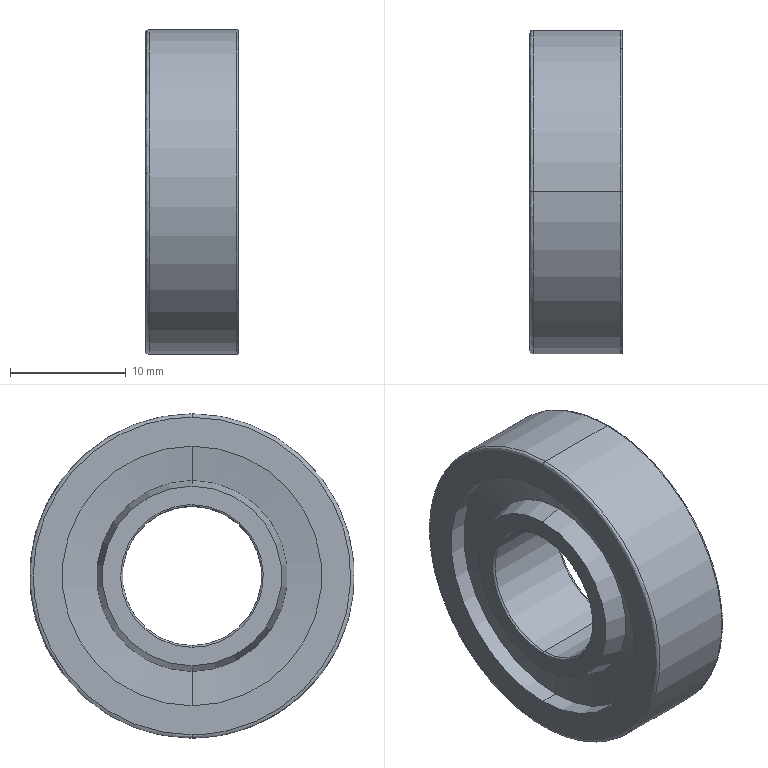Part | STEP file | b7001su | 1 solid | 28 faces | box 8 x 28 x 28 mm | volume 3327 mm3 | spline 8 | cylinder 8 | cone 8 | plane 4 | commonest cylinder face diameters 12 x2 17.6 x2 22.4 x2 28 x2